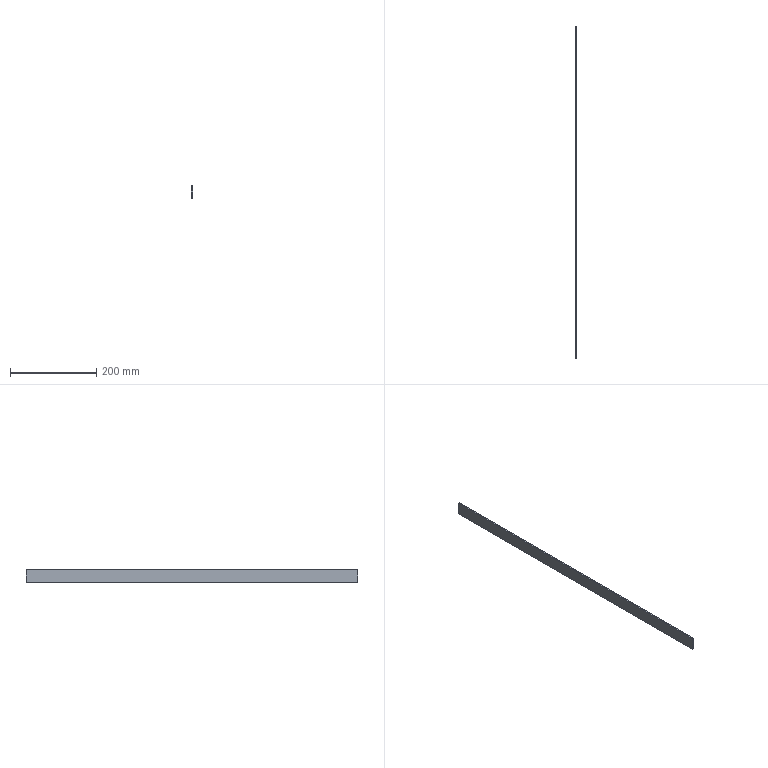Part | SolidWorks | 1 solid | 6 faces | box 3 x 770 x 30 mm | volume 69300 mm3 | plane 6
STEP:
#1=CARTESIAN_POINT('',(0.,385.,15.));
#2=VERTEX_POINT('',#1);
#3=CARTESIAN_POINT('',(0.,-385.,15.));
#4=VERTEX_POINT('',#3);
#5=CARTESIAN_POINT('',(0.,-385.,15.));
#6=DIRECTION('',(0.,-1.,0.));
#7=VECTOR('',#6,1000.);
#8=LINE('',#5,#7);
#9=EDGE_CURVE('',#2,#4,#8,.T.);
#10=ORIENTED_EDGE('',*,*,#9,.F.);
#11=CARTESIAN_POINT('',(-3.,385.,15.));
#12=VERTEX_POINT('',#11);
#13=CARTESIAN_POINT('',(-3.,385.,15.));
#14=DIRECTION('',(1.,0.,0.));
#15=VECTOR('',#14,1000.);
#16=LINE('',#13,#15);
#17=EDGE_CURVE('',#12,#2,#16,.T.);
#18=ORIENTED_EDGE('',*,*,#17,.F.);
#19=CARTESIAN_POINT('',(-3.,-385.,15.));
#20=VERTEX_POINT('',#19);
#21=CARTESIAN_POINT('',(-3.,-385.,15.));
#22=DIRECTION('',(0.,-1.,0.));
#23=VECTOR('',#22,1000.);
#24=LINE('',#21,#23);
#25=EDGE_CURVE('',#12,#20,#24,.T.);
#26=ORIENTED_EDGE('',*,*,#25,.T.);
#27=CARTESIAN_POINT('',(-3.,-385.,15.));
#28=DIRECTION('',(1.,0.,0.));
#29=VECTOR('',#28,1000.);
#30=LINE('',#27,#29);
#31=EDGE_CURVE('',#20,#4,#30,.T.);
#32=ORIENTED_EDGE('',*,*,#31,.T.);
#33=EDGE_LOOP('',(#10,#18,#26,#32));
#34=FACE_OUTER_BOUND('',#33,.T.);
#35=CARTESIAN_POINT('',(-3.,-385.,15.));
#36=DIRECTION('',(0.,0.,1.));
#37=DIRECTION('',(1.,0.,0.));
#38=AXIS2_PLACEMENT_3D('',#35,#36,#37);
#39=PLANE('',#38);
#40=ADVANCED_FACE('',(#34),#39,.T.);
#41=CARTESIAN_POINT('',(0.,385.,-15.));
#42=VERTEX_POINT('',#41);
#43=CARTESIAN_POINT('',(0.,385.,-15.));
#44=DIRECTION('',(0.,0.,1.));
#45=VECTOR('',#44,1000.);
#46=LINE('',#43,#45);
#47=EDGE_CURVE('',#42,#2,#46,.T.);
#48=ORIENTED_EDGE('',*,*,#47,.F.);
#49=CARTESIAN_POINT('',(-3.,385.,-15.));
#50=VERTEX_POINT('',#49);
#51=CARTESIAN_POINT('',(-3.,385.,-15.));
#52=DIRECTION('',(1.,0.,0.));
#53=VECTOR('',#52,1000.);
#54=LINE('',#51,#53);
#55=EDGE_CURVE('',#50,#42,#54,.T.);
#56=ORIENTED_EDGE('',*,*,#55,.F.);
#57=CARTESIAN_POINT('',(-3.,385.,-15.));
#58=DIRECTION('',(0.,0.,1.));
#59=VECTOR('',#58,1000.);
#60=LINE('',#57,#59);
#61=EDGE_CURVE('',#50,#12,#60,.T.);
#62=ORIENTED_EDGE('',*,*,#61,.T.);
#63=ORIENTED_EDGE('',*,*,#17,.T.);
#64=EDGE_LOOP('',(#48,#56,#62,#63));
#65=FACE_OUTER_BOUND('',#64,.T.);
#66=CARTESIAN_POINT('',(-3.,385.,-15.));
#67=DIRECTION('',(0.,1.,0.));
#68=DIRECTION('',(0.,0.,1.));
#69=AXIS2_PLACEMENT_3D('',#66,#67,#68);
#70=PLANE('',#69);
#71=ADVANCED_FACE('',(#65),#70,.T.);
#72=CARTESIAN_POINT('',(0.,-385.,-15.));
#73=VERTEX_POINT('',#72);
#74=CARTESIAN_POINT('',(0.,-385.,-15.));
#75=DIRECTION('',(0.,1.,0.));
#76=VECTOR('',#75,1000.);
#77=LINE('',#74,#76);
#78=EDGE_CURVE('',#73,#42,#77,.T.);
#79=ORIENTED_EDGE('',*,*,#78,.F.);
#80=CARTESIAN_POINT('',(-3.,-385.,-15.));
#81=VERTEX_POINT('',#80);
#82=CARTESIAN_POINT('',(-3.,-385.,-15.));
#83=DIRECTION('',(1.,0.,0.));
#84=VECTOR('',#83,1000.);
#85=LINE('',#82,#84);
#86=EDGE_CURVE('',#81,#73,#85,.T.);
#87=ORIENTED_EDGE('',*,*,#86,.F.);
#88=CARTESIAN_POINT('',(-3.,-385.,-15.));
#89=DIRECTION('',(0.,1.,0.));
#90=VECTOR('',#89,1000.);
#91=LINE('',#88,#90);
#92=EDGE_CURVE('',#81,#50,#91,.T.);
#93=ORIENTED_EDGE('',*,*,#92,.T.);
#94=ORIENTED_EDGE('',*,*,#55,.T.);
#95=EDGE_LOOP('',(#79,#87,#93,#94));
#96=FACE_OUTER_BOUND('',#95,.T.);
#97=CARTESIAN_POINT('',(-3.,-385.,-15.));
#98=DIRECTION('',(0.,0.,-1.));
#99=DIRECTION('',(-1.,0.,0.));
#100=AXIS2_PLACEMENT_3D('',#97,#98,#99);
#101=PLANE('',#100);
#102=ADVANCED_FACE('',(#96),#101,.T.);
#103=CARTESIAN_POINT('',(0.,-385.,-15.));
#104=DIRECTION('',(0.,0.,-1.));
#105=VECTOR('',#104,1000.);
#106=LINE('',#103,#105);
#107=EDGE_CURVE('',#4,#73,#106,.T.);
#108=ORIENTED_EDGE('',*,*,#107,.F.);
#109=ORIENTED_EDGE('',*,*,#31,.F.);
#110=CARTESIAN_POINT('',(-3.,-385.,-15.));
#111=DIRECTION('',(0.,0.,-1.));
#112=VECTOR('',#111,1000.);
#113=LINE('',#110,#112);
#114=EDGE_CURVE('',#20,#81,#113,.T.);
#115=ORIENTED_EDGE('',*,*,#114,.T.);
#116=ORIENTED_EDGE('',*,*,#86,.T.);
#117=EDGE_LOOP('',(#108,#109,#115,#116));
#118=FACE_OUTER_BOUND('',#117,.T.);
#119=CARTESIAN_POINT('',(-3.,-385.,-15.));
#120=DIRECTION('',(0.,-1.,0.));
#121=DIRECTION('',(0.,0.,-1.));
#122=AXIS2_PLACEMENT_3D('',#119,#120,#121);
#123=PLANE('',#122);
#124=ADVANCED_FACE('',(#118),#123,.T.);
#125=ORIENTED_EDGE('',*,*,#25,.F.);
#126=ORIENTED_EDGE('',*,*,#61,.F.);
#127=ORIENTED_EDGE('',*,*,#92,.F.);
#128=ORIENTED_EDGE('',*,*,#114,.F.);
#129=EDGE_LOOP('',(#125,#126,#127,#128));
#130=FACE_OUTER_BOUND('',#129,.T.);
#131=CARTESIAN_POINT('',(-3.,0.,0.));
#132=DIRECTION('',(1.,0.,0.));
#133=DIRECTION('',(0.,0.,-1.));
#134=AXIS2_PLACEMENT_3D('',#131,#132,#133);
#135=PLANE('',#134);
#136=ADVANCED_FACE('',(#130),#135,.F.);
#137=ORIENTED_EDGE('',*,*,#9,.T.);
#138=ORIENTED_EDGE('',*,*,#107,.T.);
#139=ORIENTED_EDGE('',*,*,#78,.T.);
#140=ORIENTED_EDGE('',*,*,#47,.T.);
#141=EDGE_LOOP('',(#137,#138,#139,#140));
#142=FACE_OUTER_BOUND('',#141,.T.);
#143=CARTESIAN_POINT('',(0.,0.,0.));
#144=DIRECTION('',(1.,0.,0.));
#145=DIRECTION('',(0.,0.,-1.));
#146=AXIS2_PLACEMENT_3D('',#143,#144,#145);
#147=PLANE('',#146);
#148=ADVANCED_FACE('',(#142),#147,.T.);
#149=CLOSED_SHELL('',(#40,#71,#102,#124,#136,#148));
#150=MANIFOLD_SOLID_BREP('',#149);
#151=CARTESIAN_POINT('',(0.,0.,0.));
#152=DIRECTION('',(0.,0.,1.));
#153=DIRECTION('',(1.,0.,0.));
#154=AXIS2_PLACEMENT_3D('',#151,#152,#153);
#155=(LENGTH_UNIT()NAMED_UNIT(*)SI_UNIT(.MILLI.,.METRE.));
#156=UNCERTAINTY_MEASURE_WITH_UNIT(LENGTH_MEASURE(0.00001),#155,'','');
#157=(NAMED_UNIT(*)PLANE_ANGLE_UNIT()SI_UNIT($,.RADIAN.));
#158=(NAMED_UNIT(*)SI_UNIT($,.STERADIAN.)SOLID_ANGLE_UNIT());
#159=(GEOMETRIC_REPRESENTATION_CONTEXT(3)GLOBAL_UNCERTAINTY_ASSIGNED_CONTEXT((#156))GLOBAL_UNIT_ASSIGNED_CONTEXT((#155,#157,#158))REPRESENTATION_CONTEXT('',''));
#160=ADVANCED_BREP_SHAPE_REPRESENTATION('',(#150,#154),#159);